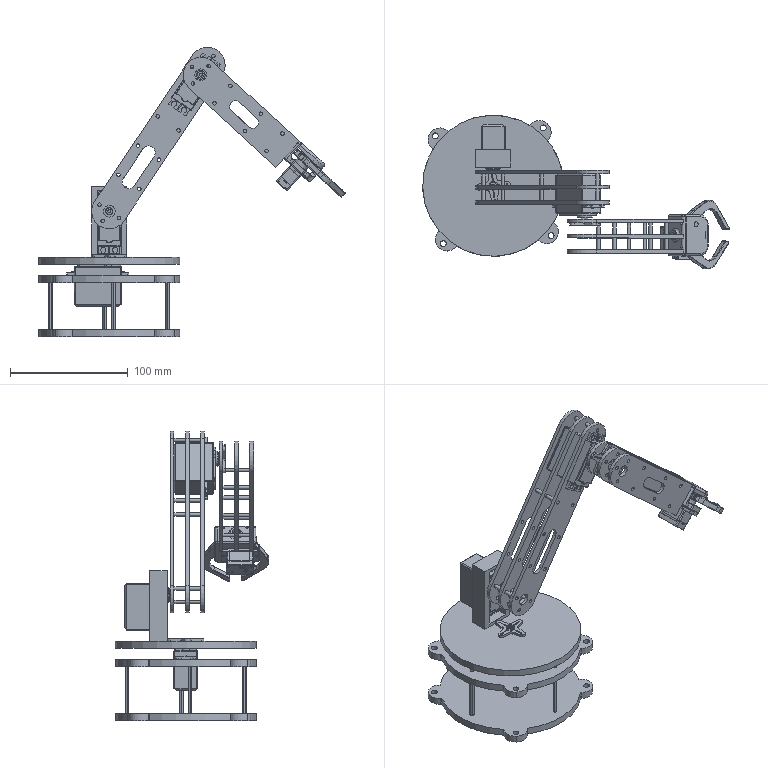Part | STEP file | Assem1 | 57 solids | 2537 faces | box 260.751 x 130.76 x 246.419 mm | volume 394553 mm3 | plane 1236 | cylinder 840 | torus 222 | spline 167 | sphere 68 | cone 4 | commonest cylinder face diameters 6 x183 1 x121 3 x85 5 x67 4.9 x60 2 x44